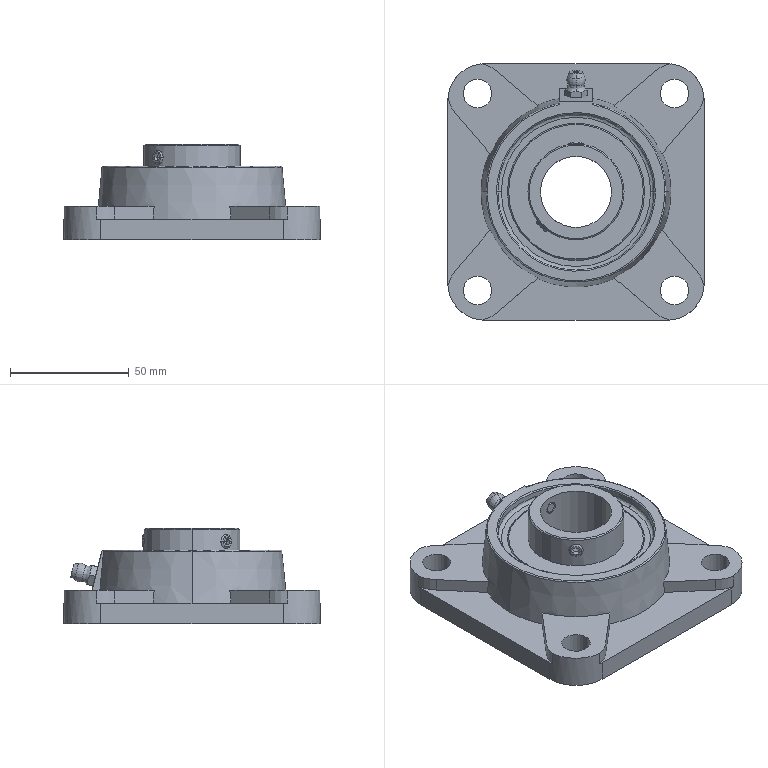Part | SolidWorks | 3 solids | 151 faces | box 108 x 108 x 40.2 mm | volume 171689 mm3 | plane 66 | cylinder 42 | cone 27 | spline 14 | torus 2 | commonest cylinder face diameters 12 x8 25 x8 5.188 x4 6 x4 31 x4 40.5 x4